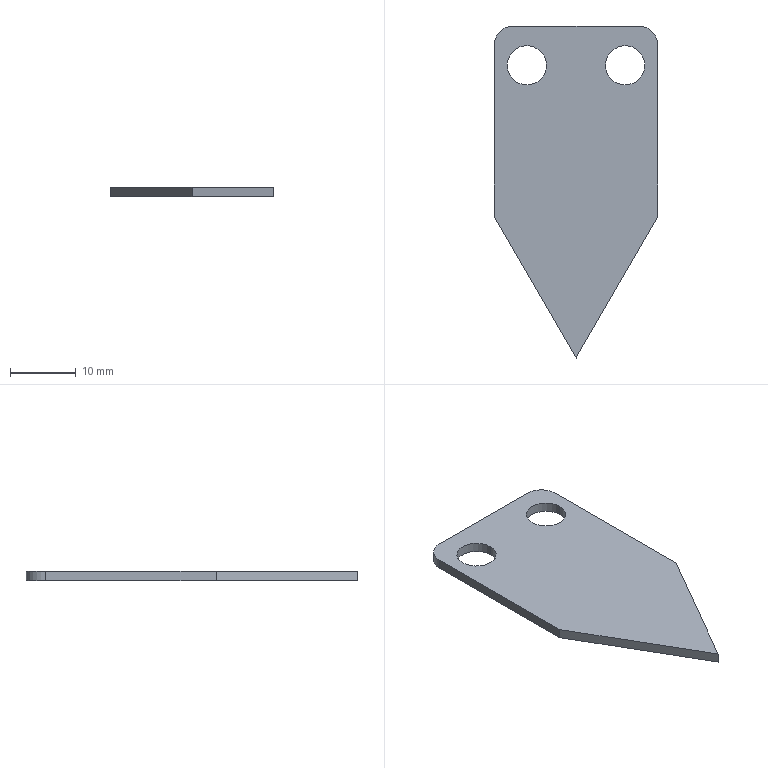Part | SolidWorks | features Extrusion 1, Fillet 1, HoleWzd 1 | 1 solid | 13 faces | box 25 x 50.651 x 1.5 mm | volume 1403 mm3 | plane 7 | cylinder 6 | commonest cylinder face diameters 6 x6
STEP:
#1=CARTESIAN_POINT('',(-10.5,-6.,0.));
#2=VERTEX_POINT('',#1);
#3=CARTESIAN_POINT('',(-4.5,-6.,0.));
#4=VERTEX_POINT('',#3);
#5=CARTESIAN_POINT('',(-7.5,-6.,0.));
#6=DIRECTION('',(0.,0.,1.));
#7=DIRECTION('',(1.,0.,0.));
#8=AXIS2_PLACEMENT_3D('',#5,#6,#7);
#9=CIRCLE('',#8,3.);
#10=EDGE_CURVE('',#2,#4,#9,.T.);
#11=ORIENTED_EDGE('',*,*,#10,.F.);
#12=CARTESIAN_POINT('',(-10.5,-6.,1.5));
#13=VERTEX_POINT('',#12);
#14=CARTESIAN_POINT('',(-10.5,-6.,1.5));
#15=DIRECTION('',(0.,0.,1.));
#16=VECTOR('',#15,1000.);
#17=LINE('',#14,#16);
#18=EDGE_CURVE('',#2,#13,#17,.T.);
#19=ORIENTED_EDGE('',*,*,#18,.T.);
#20=CARTESIAN_POINT('',(-4.5,-6.,1.5));
#21=VERTEX_POINT('',#20);
#22=CARTESIAN_POINT('',(-7.5,-6.,1.5));
#23=DIRECTION('',(0.,0.,1.));
#24=DIRECTION('',(1.,0.,0.));
#25=AXIS2_PLACEMENT_3D('',#22,#23,#24);
#26=CIRCLE('',#25,3.);
#27=EDGE_CURVE('',#13,#21,#26,.T.);
#28=ORIENTED_EDGE('',*,*,#27,.T.);
#29=CARTESIAN_POINT('',(-4.5,-6.,1.5));
#30=DIRECTION('',(0.,0.,1.));
#31=VECTOR('',#30,1000.);
#32=LINE('',#29,#31);
#33=EDGE_CURVE('',#4,#21,#32,.T.);
#34=ORIENTED_EDGE('',*,*,#33,.F.);
#35=EDGE_LOOP('',(#11,#19,#28,#34));
#36=FACE_OUTER_BOUND('',#35,.T.);
#37=CARTESIAN_POINT('',(-7.5,-6.,1.5));
#38=DIRECTION('',(0.,0.,1.));
#39=DIRECTION('',(1.,0.,0.));
#40=AXIS2_PLACEMENT_3D('',#37,#38,#39);
#41=CYLINDRICAL_SURFACE('',#40,3.);
#42=ADVANCED_FACE('',(#36),#41,.F.);
#43=CARTESIAN_POINT('',(4.5,-6.,0.));
#44=VERTEX_POINT('',#43);
#45=CARTESIAN_POINT('',(10.5,-6.,0.));
#46=VERTEX_POINT('',#45);
#47=CARTESIAN_POINT('',(7.5,-6.,0.));
#48=DIRECTION('',(0.,0.,1.));
#49=DIRECTION('',(1.,0.,0.));
#50=AXIS2_PLACEMENT_3D('',#47,#48,#49);
#51=CIRCLE('',#50,3.);
#52=EDGE_CURVE('',#44,#46,#51,.T.);
#53=ORIENTED_EDGE('',*,*,#52,.F.);
#54=CARTESIAN_POINT('',(4.5,-6.,1.5));
#55=VERTEX_POINT('',#54);
#56=CARTESIAN_POINT('',(4.5,-6.,1.5));
#57=DIRECTION('',(0.,0.,1.));
#58=VECTOR('',#57,1000.);
#59=LINE('',#56,#58);
#60=EDGE_CURVE('',#44,#55,#59,.T.);
#61=ORIENTED_EDGE('',*,*,#60,.T.);
#62=CARTESIAN_POINT('',(10.5,-6.,1.5));
#63=VERTEX_POINT('',#62);
#64=CARTESIAN_POINT('',(7.5,-6.,1.5));
#65=DIRECTION('',(0.,0.,1.));
#66=DIRECTION('',(1.,0.,0.));
#67=AXIS2_PLACEMENT_3D('',#64,#65,#66);
#68=CIRCLE('',#67,3.);
#69=EDGE_CURVE('',#55,#63,#68,.T.);
#70=ORIENTED_EDGE('',*,*,#69,.T.);
#71=CARTESIAN_POINT('',(10.5,-6.,1.5));
#72=DIRECTION('',(0.,0.,1.));
#73=VECTOR('',#72,1000.);
#74=LINE('',#71,#73);
#75=EDGE_CURVE('',#46,#63,#74,.T.);
#76=ORIENTED_EDGE('',*,*,#75,.F.);
#77=EDGE_LOOP('',(#53,#61,#70,#76));
#78=FACE_OUTER_BOUND('',#77,.T.);
#79=CARTESIAN_POINT('',(7.5,-6.,1.5));
#80=DIRECTION('',(0.,0.,1.));
#81=DIRECTION('',(1.,0.,0.));
#82=AXIS2_PLACEMENT_3D('',#79,#80,#81);
#83=CYLINDRICAL_SURFACE('',#82,3.);
#84=ADVANCED_FACE('',(#78),#83,.F.);
#85=CARTESIAN_POINT('',(-12.5,-3.,1.5));
#86=VERTEX_POINT('',#85);
#87=CARTESIAN_POINT('',(-12.5,-29.,1.5));
#88=VERTEX_POINT('',#87);
#89=CARTESIAN_POINT('',(-12.5,-29.,1.5));
#90=DIRECTION('',(0.,-1.,0.));
#91=VECTOR('',#90,1000.);
#92=LINE('',#89,#91);
#93=EDGE_CURVE('',#86,#88,#92,.T.);
#94=ORIENTED_EDGE('',*,*,#93,.F.);
#95=CARTESIAN_POINT('',(-12.5,-3.,0.));
#96=VERTEX_POINT('',#95);
#97=CARTESIAN_POINT('',(-12.5,-3.,1.5));
#98=DIRECTION('',(0.,0.,-1.));
#99=VECTOR('',#98,1000.);
#100=LINE('',#97,#99);
#101=EDGE_CURVE('',#86,#96,#100,.T.);
#102=ORIENTED_EDGE('',*,*,#101,.T.);
#103=CARTESIAN_POINT('',(-12.5,-29.,0.));
#104=VERTEX_POINT('',#103);
#105=CARTESIAN_POINT('',(-12.5,-29.,0.));
#106=DIRECTION('',(0.,-1.,0.));
#107=VECTOR('',#106,1000.);
#108=LINE('',#105,#107);
#109=EDGE_CURVE('',#96,#104,#108,.T.);
#110=ORIENTED_EDGE('',*,*,#109,.T.);
#111=CARTESIAN_POINT('',(-12.5,-29.,1.5));
#112=DIRECTION('',(0.,0.,-1.));
#113=VECTOR('',#112,1000.);
#114=LINE('',#111,#113);
#115=EDGE_CURVE('',#88,#104,#114,.T.);
#116=ORIENTED_EDGE('',*,*,#115,.F.);
#117=EDGE_LOOP('',(#94,#102,#110,#116));
#118=FACE_OUTER_BOUND('',#117,.T.);
#119=CARTESIAN_POINT('',(-12.5,-29.,1.5));
#120=DIRECTION('',(1.,0.,0.));
#121=DIRECTION('',(0.,1.,0.));
#122=AXIS2_PLACEMENT_3D('',#119,#120,#121);
#123=PLANE('',#122);
#124=ADVANCED_FACE('',(#118),#123,.F.);
#125=CARTESIAN_POINT('',(0.,-50.651,0.));
#126=VERTEX_POINT('',#125);
#127=CARTESIAN_POINT('',(-12.5,-29.,0.));
#128=DIRECTION('',(0.5,-0.866,0.));
#129=VECTOR('',#128,1000.);
#130=LINE('',#127,#129);
#131=EDGE_CURVE('',#104,#126,#130,.T.);
#132=ORIENTED_EDGE('',*,*,#131,.T.);
#133=CARTESIAN_POINT('',(0.,-50.651,1.5));
#134=VERTEX_POINT('',#133);
#135=CARTESIAN_POINT('',(0.,-50.651,1.5));
#136=DIRECTION('',(0.,0.,-1.));
#137=VECTOR('',#136,1000.);
#138=LINE('',#135,#137);
#139=EDGE_CURVE('',#134,#126,#138,.T.);
#140=ORIENTED_EDGE('',*,*,#139,.F.);
#141=CARTESIAN_POINT('',(-12.5,-29.,1.5));
#142=DIRECTION('',(0.5,-0.866,0.));
#143=VECTOR('',#142,1000.);
#144=LINE('',#141,#143);
#145=EDGE_CURVE('',#88,#134,#144,.T.);
#146=ORIENTED_EDGE('',*,*,#145,.F.);
#147=ORIENTED_EDGE('',*,*,#115,.T.);
#148=EDGE_LOOP('',(#132,#140,#146,#147));
#149=FACE_OUTER_BOUND('',#148,.T.);
#150=CARTESIAN_POINT('',(-12.5,-29.,1.5));
#151=DIRECTION('',(0.866,0.5,0.));
#152=DIRECTION('',(-0.5,0.866,0.));
#153=AXIS2_PLACEMENT_3D('',#150,#151,#152);
#154=PLANE('',#153);
#155=ADVANCED_FACE('',(#149),#154,.F.);
#156=CARTESIAN_POINT('',(12.5,-29.,0.));
#157=VERTEX_POINT('',#156);
#158=CARTESIAN_POINT('',(0.,-50.651,0.));
#159=DIRECTION('',(0.5,0.866,0.));
#160=VECTOR('',#159,1000.);
#161=LINE('',#158,#160);
#162=EDGE_CURVE('',#126,#157,#161,.T.);
#163=ORIENTED_EDGE('',*,*,#162,.T.);
#164=CARTESIAN_POINT('',(12.5,-29.,1.5));
#165=VERTEX_POINT('',#164);
#166=CARTESIAN_POINT('',(12.5,-29.,1.5));
#167=DIRECTION('',(0.,0.,-1.));
#168=VECTOR('',#167,1000.);
#169=LINE('',#166,#168);
#170=EDGE_CURVE('',#165,#157,#169,.T.);
#171=ORIENTED_EDGE('',*,*,#170,.F.);
#172=CARTESIAN_POINT('',(0.,-50.651,1.5));
#173=DIRECTION('',(0.5,0.866,0.));
#174=VECTOR('',#173,1000.);
#175=LINE('',#172,#174);
#176=EDGE_CURVE('',#134,#165,#175,.T.);
#177=ORIENTED_EDGE('',*,*,#176,.F.);
#178=ORIENTED_EDGE('',*,*,#139,.T.);
#179=EDGE_LOOP('',(#163,#171,#177,#178));
#180=FACE_OUTER_BOUND('',#179,.T.);
#181=CARTESIAN_POINT('',(0.,-50.651,1.5));
#182=DIRECTION('',(-0.866,0.5,0.));
#183=DIRECTION('',(-0.5,-0.866,0.));
#184=AXIS2_PLACEMENT_3D('',#181,#182,#183);
#185=PLANE('',#184);
#186=ADVANCED_FACE('',(#180),#185,.F.);
#187=CARTESIAN_POINT('',(12.5,-3.,0.));
#188=VERTEX_POINT('',#187);
#189=CARTESIAN_POINT('',(12.5,0.,0.));
#190=DIRECTION('',(0.,1.,0.));
#191=VECTOR('',#190,1000.);
#192=LINE('',#189,#191);
#193=EDGE_CURVE('',#157,#188,#192,.T.);
#194=ORIENTED_EDGE('',*,*,#193,.T.);
#195=CARTESIAN_POINT('',(12.5,-3.,1.5));
#196=VERTEX_POINT('',#195);
#197=CARTESIAN_POINT('',(12.5,-3.,1.5));
#198=DIRECTION('',(0.,0.,1.));
#199=VECTOR('',#198,1000.);
#200=LINE('',#197,#199);
#201=EDGE_CURVE('',#188,#196,#200,.T.);
#202=ORIENTED_EDGE('',*,*,#201,.T.);
#203=CARTESIAN_POINT('',(12.5,0.,1.5));
#204=DIRECTION('',(0.,1.,0.));
#205=VECTOR('',#204,1000.);
#206=LINE('',#203,#205);
#207=EDGE_CURVE('',#165,#196,#206,.T.);
#208=ORIENTED_EDGE('',*,*,#207,.F.);
#209=ORIENTED_EDGE('',*,*,#170,.T.);
#210=EDGE_LOOP('',(#194,#202,#208,#209));
#211=FACE_OUTER_BOUND('',#210,.T.);
#212=CARTESIAN_POINT('',(12.5,0.,1.5));
#213=DIRECTION('',(-1.,0.,0.));
#214=DIRECTION('',(0.,-1.,0.));
#215=AXIS2_PLACEMENT_3D('',#212,#213,#214);
#216=PLANE('',#215);
#217=ADVANCED_FACE('',(#211),#216,.F.);
#218=CARTESIAN_POINT('',(9.5,0.,1.5));
#219=VERTEX_POINT('',#218);
#220=CARTESIAN_POINT('',(-9.5,0.,1.5));
#221=VERTEX_POINT('',#220);
#222=CARTESIAN_POINT('',(-12.5,0.,1.5));
#223=DIRECTION('',(-1.,0.,0.));
#224=VECTOR('',#223,1000.);
#225=LINE('',#222,#224);
#226=EDGE_CURVE('',#219,#221,#225,.T.);
#227=ORIENTED_EDGE('',*,*,#226,.F.);
#228=CARTESIAN_POINT('',(9.5,0.,0.));
#229=VERTEX_POINT('',#228);
#230=CARTESIAN_POINT('',(9.5,0.,1.5));
#231=DIRECTION('',(0.,0.,-1.));
#232=VECTOR('',#231,1000.);
#233=LINE('',#230,#232);
#234=EDGE_CURVE('',#219,#229,#233,.T.);
#235=ORIENTED_EDGE('',*,*,#234,.T.);
#236=CARTESIAN_POINT('',(-9.5,0.,0.));
#237=VERTEX_POINT('',#236);
#238=CARTESIAN_POINT('',(-12.5,0.,0.));
#239=DIRECTION('',(-1.,0.,0.));
#240=VECTOR('',#239,1000.);
#241=LINE('',#238,#240);
#242=EDGE_CURVE('',#229,#237,#241,.T.);
#243=ORIENTED_EDGE('',*,*,#242,.T.);
#244=CARTESIAN_POINT('',(-9.5,0.,1.5));
#245=DIRECTION('',(0.,0.,1.));
#246=VECTOR('',#245,1000.);
#247=LINE('',#244,#246);
#248=EDGE_CURVE('',#237,#221,#247,.T.);
#249=ORIENTED_EDGE('',*,*,#248,.T.);
#250=EDGE_LOOP('',(#227,#235,#243,#249));
#251=FACE_OUTER_BOUND('',#250,.T.);
#252=CARTESIAN_POINT('',(-12.5,0.,1.5));
#253=DIRECTION('',(0.,-1.,0.));
#254=DIRECTION('',(1.,0.,0.));
#255=AXIS2_PLACEMENT_3D('',#252,#253,#254);
#256=PLANE('',#255);
#257=ADVANCED_FACE('',(#251),#256,.F.);
#258=CARTESIAN_POINT('',(-7.5,-6.,1.5));
#259=DIRECTION('',(0.,0.,1.));
#260=DIRECTION('',(1.,0.,0.));
#261=AXIS2_PLACEMENT_3D('',#258,#259,#260);
#262=CIRCLE('',#261,3.);
#263=EDGE_CURVE('',#21,#13,#262,.T.);
#264=ORIENTED_EDGE('',*,*,#263,.F.);
#265=ORIENTED_EDGE('',*,*,#27,.F.);
#266=EDGE_LOOP('',(#264,#265));
#267=FACE_BOUND('',#266,.T.);
#268=CARTESIAN_POINT('',(7.5,-6.,1.5));
#269=DIRECTION('',(0.,0.,1.));
#270=DIRECTION('',(1.,0.,0.));
#271=AXIS2_PLACEMENT_3D('',#268,#269,#270);
#272=CIRCLE('',#271,3.);
#273=EDGE_CURVE('',#63,#55,#272,.T.);
#274=ORIENTED_EDGE('',*,*,#273,.F.);
#275=ORIENTED_EDGE('',*,*,#69,.F.);
#276=EDGE_LOOP('',(#274,#275));
#277=FACE_BOUND('',#276,.T.);
#278=ORIENTED_EDGE('',*,*,#207,.T.);
#279=CARTESIAN_POINT('',(9.5,-3.,1.5));
#280=DIRECTION('',(0.,0.,1.));
#281=DIRECTION('',(-1.,0.,0.));
#282=AXIS2_PLACEMENT_3D('',#279,#280,#281);
#283=CIRCLE('',#282,3.);
#284=EDGE_CURVE('',#196,#219,#283,.T.);
#285=ORIENTED_EDGE('',*,*,#284,.T.);
#286=ORIENTED_EDGE('',*,*,#226,.T.);
#287=CARTESIAN_POINT('',(-9.5,-3.,1.5));
#288=DIRECTION('',(0.,0.,1.));
#289=DIRECTION('',(-1.,0.,0.));
#290=AXIS2_PLACEMENT_3D('',#287,#288,#289);
#291=CIRCLE('',#290,3.);
#292=EDGE_CURVE('',#221,#86,#291,.T.);
#293=ORIENTED_EDGE('',*,*,#292,.T.);
#294=ORIENTED_EDGE('',*,*,#93,.T.);
#295=ORIENTED_EDGE('',*,*,#145,.T.);
#296=ORIENTED_EDGE('',*,*,#176,.T.);
#297=EDGE_LOOP('',(#278,#285,#286,#293,#294,#295,#296));
#298=FACE_OUTER_BOUND('',#297,.T.);
#299=CARTESIAN_POINT('',(0.,0.,1.5));
#300=DIRECTION('',(0.,0.,-1.));
#301=DIRECTION('',(-1.,0.,0.));
#302=AXIS2_PLACEMENT_3D('',#299,#300,#301);
#303=PLANE('',#302);
#304=ADVANCED_FACE('',(#267,#277,#298),#303,.F.);
#305=CARTESIAN_POINT('',(-7.5,-6.,0.));
#306=DIRECTION('',(0.,0.,1.));
#307=DIRECTION('',(1.,0.,0.));
#308=AXIS2_PLACEMENT_3D('',#305,#306,#307);
#309=CIRCLE('',#308,3.);
#310=EDGE_CURVE('',#4,#2,#309,.T.);
#311=ORIENTED_EDGE('',*,*,#310,.T.);
#312=ORIENTED_EDGE('',*,*,#10,.T.);
#313=EDGE_LOOP('',(#311,#312));
#314=FACE_BOUND('',#313,.T.);
#315=CARTESIAN_POINT('',(7.5,-6.,0.));
#316=DIRECTION('',(0.,0.,1.));
#317=DIRECTION('',(1.,0.,0.));
#318=AXIS2_PLACEMENT_3D('',#315,#316,#317);
#319=CIRCLE('',#318,3.);
#320=EDGE_CURVE('',#46,#44,#319,.T.);
#321=ORIENTED_EDGE('',*,*,#320,.T.);
#322=ORIENTED_EDGE('',*,*,#52,.T.);
#323=EDGE_LOOP('',(#321,#322));
#324=FACE_BOUND('',#323,.T.);
#325=ORIENTED_EDGE('',*,*,#242,.F.);
#326=CARTESIAN_POINT('',(9.5,-3.,0.));
#327=DIRECTION('',(0.,0.,-1.));
#328=DIRECTION('',(-1.,0.,0.));
#329=AXIS2_PLACEMENT_3D('',#326,#327,#328);
#330=CIRCLE('',#329,3.);
#331=EDGE_CURVE('',#229,#188,#330,.T.);
#332=ORIENTED_EDGE('',*,*,#331,.T.);
#333=ORIENTED_EDGE('',*,*,#193,.F.);
#334=ORIENTED_EDGE('',*,*,#162,.F.);
#335=ORIENTED_EDGE('',*,*,#131,.F.);
#336=ORIENTED_EDGE('',*,*,#109,.F.);
#337=CARTESIAN_POINT('',(-9.5,-3.,0.));
#338=DIRECTION('',(0.,0.,-1.));
#339=DIRECTION('',(-1.,0.,0.));
#340=AXIS2_PLACEMENT_3D('',#337,#338,#339);
#341=CIRCLE('',#340,3.);
#342=EDGE_CURVE('',#96,#237,#341,.T.);
#343=ORIENTED_EDGE('',*,*,#342,.T.);
#344=EDGE_LOOP('',(#325,#332,#333,#334,#335,#336,#343));
#345=FACE_OUTER_BOUND('',#344,.T.);
#346=CARTESIAN_POINT('',(0.,0.,0.));
#347=DIRECTION('',(0.,0.,-1.));
#348=DIRECTION('',(-1.,0.,0.));
#349=AXIS2_PLACEMENT_3D('',#346,#347,#348);
#350=PLANE('',#349);
#351=ADVANCED_FACE('',(#314,#324,#345),#350,.T.);
#352=ORIENTED_EDGE('',*,*,#60,.F.);
#353=ORIENTED_EDGE('',*,*,#320,.F.);
#354=ORIENTED_EDGE('',*,*,#75,.T.);
#355=ORIENTED_EDGE('',*,*,#273,.T.);
#356=EDGE_LOOP('',(#352,#353,#354,#355));
#357=FACE_OUTER_BOUND('',#356,.T.);
#358=CARTESIAN_POINT('',(7.5,-6.,1.5));
#359=DIRECTION('',(0.,0.,1.));
#360=DIRECTION('',(1.,0.,0.));
#361=AXIS2_PLACEMENT_3D('',#358,#359,#360);
#362=CYLINDRICAL_SURFACE('',#361,3.);
#363=ADVANCED_FACE('',(#357),#362,.F.);
#364=ORIENTED_EDGE('',*,*,#18,.F.);
#365=ORIENTED_EDGE('',*,*,#310,.F.);
#366=ORIENTED_EDGE('',*,*,#33,.T.);
#367=ORIENTED_EDGE('',*,*,#263,.T.);
#368=EDGE_LOOP('',(#364,#365,#366,#367));
#369=FACE_OUTER_BOUND('',#368,.T.);
#370=CARTESIAN_POINT('',(-7.5,-6.,1.5));
#371=DIRECTION('',(0.,0.,1.));
#372=DIRECTION('',(1.,0.,0.));
#373=AXIS2_PLACEMENT_3D('',#370,#371,#372);
#374=CYLINDRICAL_SURFACE('',#373,3.);
#375=ADVANCED_FACE('',(#369),#374,.F.);
#376=ORIENTED_EDGE('',*,*,#284,.F.);
#377=ORIENTED_EDGE('',*,*,#201,.F.);
#378=ORIENTED_EDGE('',*,*,#331,.F.);
#379=ORIENTED_EDGE('',*,*,#234,.F.);
#380=EDGE_LOOP('',(#376,#377,#378,#379));
#381=FACE_OUTER_BOUND('',#380,.T.);
#382=CARTESIAN_POINT('',(9.5,-3.,1.5));
#383=DIRECTION('',(0.,0.,-1.));
#384=DIRECTION('',(-1.,0.,0.));
#385=AXIS2_PLACEMENT_3D('',#382,#383,#384);
#386=CYLINDRICAL_SURFACE('',#385,3.);
#387=ADVANCED_FACE('',(#381),#386,.T.);
#388=ORIENTED_EDGE('',*,*,#292,.F.);
#389=ORIENTED_EDGE('',*,*,#248,.F.);
#390=ORIENTED_EDGE('',*,*,#342,.F.);
#391=ORIENTED_EDGE('',*,*,#101,.F.);
#392=EDGE_LOOP('',(#388,#389,#390,#391));
#393=FACE_OUTER_BOUND('',#392,.T.);
#394=CARTESIAN_POINT('',(-9.5,-3.,1.5));
#395=DIRECTION('',(0.,0.,-1.));
#396=DIRECTION('',(-1.,0.,0.));
#397=AXIS2_PLACEMENT_3D('',#394,#395,#396);
#398=CYLINDRICAL_SURFACE('',#397,3.);
#399=ADVANCED_FACE('',(#393),#398,.T.);
#400=CLOSED_SHELL('',(#42,#84,#124,#155,#186,#217,#257,#304,#351,#363,#375,#387,#399));
#401=MANIFOLD_SOLID_BREP('',#400);
#402=CARTESIAN_POINT('',(0.,0.,0.));
#403=DIRECTION('',(0.,0.,1.));
#404=DIRECTION('',(1.,0.,0.));
#405=AXIS2_PLACEMENT_3D('',#402,#403,#404);
#406=(LENGTH_UNIT()NAMED_UNIT(*)SI_UNIT(.MILLI.,.METRE.));
#407=UNCERTAINTY_MEASURE_WITH_UNIT(LENGTH_MEASURE(0.00001),#406,'','');
#408=(NAMED_UNIT(*)PLANE_ANGLE_UNIT()SI_UNIT($,.RADIAN.));
#409=(NAMED_UNIT(*)SI_UNIT($,.STERADIAN.)SOLID_ANGLE_UNIT());
#410=(GEOMETRIC_REPRESENTATION_CONTEXT(3)GLOBAL_UNCERTAINTY_ASSIGNED_CONTEXT((#407))GLOBAL_UNIT_ASSIGNED_CONTEXT((#406,#408,#409))REPRESENTATION_CONTEXT('',''));
#411=ADVANCED_BREP_SHAPE_REPRESENTATION('',(#401,#405),#410);